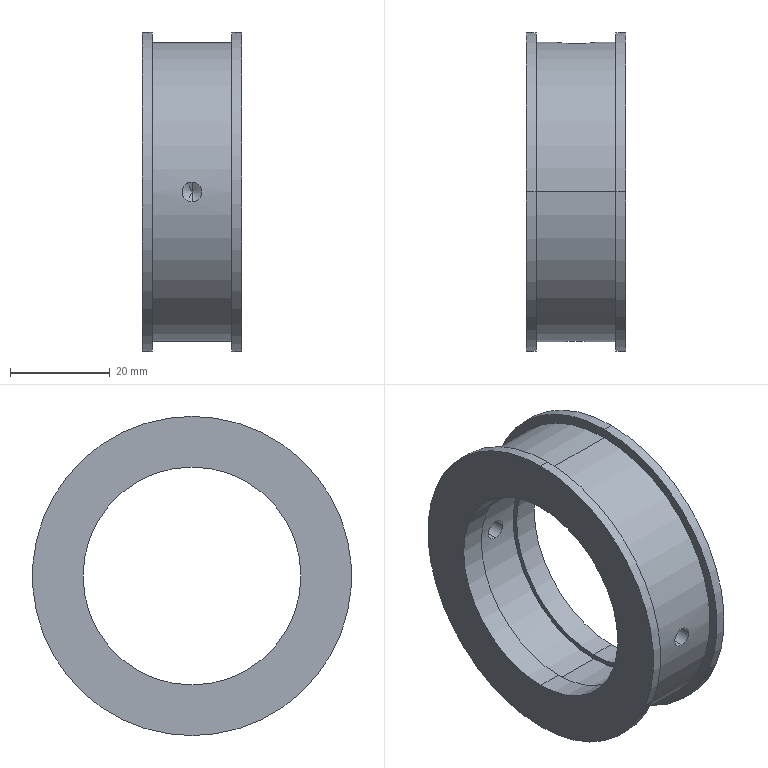Part | SolidWorks | features HoleWzd 3, Fillet 2, Revolution 1 | 1 solid | 31 faces | box 20 x 64 x 64 mm | volume 26515 mm3 | cylinder 18 | plane 7 | torus 2 | spline 2 | cone 2 | commonest cylinder face diameters 4 x4 43.7 x4 64 x4 7.5 x2 45.7 x2 60 x2
STEP:
#1=CARTESIAN_POINT('',(1.61,28.8,3.75));
#2=VERTEX_POINT('',#1);
#3=CARTESIAN_POINT('',(1.61,28.8,-3.75));
#4=VERTEX_POINT('',#3);
#5=CARTESIAN_POINT('',(1.61,28.8,0.));
#6=DIRECTION('',(0.,-1.,0.));
#7=DIRECTION('',(0.,0.,-1.));
#8=AXIS2_PLACEMENT_3D('',#5,#6,#7);
#9=CIRCLE('',#8,3.75);
#10=EDGE_CURVE('',#2,#4,#9,.T.);
#11=ORIENTED_EDGE('',*,*,#10,.F.);
#12=CARTESIAN_POINT('',(1.61,28.5,3.45));
#13=VERTEX_POINT('',#12);
#14=CARTESIAN_POINT('',(1.61,28.8,3.45));
#15=DIRECTION('',(1.,0.,0.));
#16=DIRECTION('',(0.,0.,-1.));
#17=AXIS2_PLACEMENT_3D('',#14,#15,#16);
#18=CIRCLE('',#17,0.3);
#19=EDGE_CURVE('',#2,#13,#18,.T.);
#20=ORIENTED_EDGE('',*,*,#19,.T.);
#21=CARTESIAN_POINT('',(1.61,28.5,-3.45));
#22=VERTEX_POINT('',#21);
#23=CARTESIAN_POINT('',(1.61,28.5,0.));
#24=DIRECTION('',(0.,1.,0.));
#25=DIRECTION('',(0.,0.,-1.));
#26=AXIS2_PLACEMENT_3D('',#23,#24,#25);
#27=CIRCLE('',#26,3.45);
#28=EDGE_CURVE('',#22,#13,#27,.T.);
#29=ORIENTED_EDGE('',*,*,#28,.F.);
#30=CARTESIAN_POINT('',(1.61,28.8,-3.45));
#31=DIRECTION('',(-1.,0.,0.));
#32=DIRECTION('',(0.,0.,1.));
#33=AXIS2_PLACEMENT_3D('',#30,#31,#32);
#34=CIRCLE('',#33,0.3);
#35=EDGE_CURVE('',#4,#22,#34,.T.);
#36=ORIENTED_EDGE('',*,*,#35,.F.);
#37=EDGE_LOOP('',(#11,#20,#29,#36));
#38=FACE_OUTER_BOUND('',#37,.T.);
#39=CARTESIAN_POINT('',(1.61,28.8,0.));
#40=DIRECTION('',(0.,-1.,0.));
#41=DIRECTION('',(0.,0.,-1.));
#42=AXIS2_PLACEMENT_3D('',#39,#40,#41);
#43=TOROIDAL_SURFACE('',#42,3.45,0.3);
#44=ADVANCED_FACE('',(#38),#43,.F.);
#45=CARTESIAN_POINT('',(0.7576,29.551,-3.652));
#46=VERTEX_POINT('',#45);
#47=CARTESIAN_POINT('',(1.61,29.537,3.75));
#48=VERTEX_POINT('',#47);
#49=CARTESIAN_POINT('',(0.7576,29.551,-3.652));
#50=CARTESIAN_POINT('',(0.5354,29.558,-3.6));
#51=CARTESIAN_POINT('',(0.3161,29.568,-3.527));
#52=CARTESIAN_POINT('',(-0.1007,29.591,-3.345));
#53=CARTESIAN_POINT('',(-0.2989,29.605,-3.236));
#54=CARTESIAN_POINT('',(-0.6749,29.634,-2.982));
#55=CARTESIAN_POINT('',(-0.8539,29.65,-2.836));
#56=CARTESIAN_POINT('',(-1.178,29.682,-2.518));
#57=CARTESIAN_POINT('',(-1.324,29.698,-2.346));
#58=CARTESIAN_POINT('',(-1.586,29.728,-1.974));
#59=CARTESIAN_POINT('',(-1.701,29.742,-1.774));
#60=CARTESIAN_POINT('',(-1.891,29.766,-1.363));
#61=CARTESIAN_POINT('',(-1.967,29.776,-1.149));
#62=CARTESIAN_POINT('',(-2.08,29.792,-0.7059));
#63=CARTESIAN_POINT('',(-2.116,29.797,-0.479));
#64=CARTESIAN_POINT('',(-2.146,29.801,-0.02683));
#65=CARTESIAN_POINT('',(-2.141,29.8,0.2003));
#66=CARTESIAN_POINT('',(-2.089,29.793,0.6567));
#67=CARTESIAN_POINT('',(-2.042,29.786,0.8794));
#68=CARTESIAN_POINT('',(-1.91,29.769,1.312));
#69=CARTESIAN_POINT('',(-1.823,29.757,1.524));
#70=CARTESIAN_POINT('',(-1.613,29.731,1.93));
#71=CARTESIAN_POINT('',(-1.491,29.717,2.121));
#72=CARTESIAN_POINT('',(-1.213,29.686,2.478));
#73=CARTESIAN_POINT('',(-1.056,29.67,2.647));
#74=CARTESIAN_POINT('',(-0.7163,29.638,2.95));
#75=CARTESIAN_POINT('',(-0.5345,29.623,3.084));
#76=CARTESIAN_POINT('',(-0.1474,29.594,3.32));
#77=CARTESIAN_POINT('',(0.06009,29.581,3.422));
#78=CARTESIAN_POINT('',(0.4848,29.56,3.584));
#79=CARTESIAN_POINT('',(0.7028,29.552,3.646));
#80=CARTESIAN_POINT('',(1.15,29.54,3.729));
#81=CARTESIAN_POINT('',(1.38,29.537,3.75));
#82=CARTESIAN_POINT('',(1.61,29.537,3.75));
#83=B_SPLINE_CURVE_WITH_KNOTS('',3,(#49,#50,#51,#52,#53,#54,#55,#56,#57,#58,#59,#60,#61,#62,#63,#64,#65,#66,#67,#68,#69,#70,#71,#72,#73,#74,#75,#76,#77,#78,#79,#80,#81,#82),.UNSPECIFIED.,.F.,.F.,(4,2,2,2,2,2,2,2,2,2,2,2,2,2,2,2,4),(0.01269,0.01337,0.01406,0.01474,0.01543,0.01611,0.0168,0.01748,0.01817,0.01885,0.01954,0.02022,0.02091,0.02159,0.02228,0.02296,0.02365),.UNSPECIFIED.);
#84=EDGE_CURVE('',#46,#48,#83,.T.);
#85=ORIENTED_EDGE('',*,*,#84,.F.);
#86=CARTESIAN_POINT('',(0.7121,29.749,-3.872));
#87=VERTEX_POINT('',#86);
#88=CARTESIAN_POINT('',(0.7121,29.551,-3.847));
#89=DIRECTION('',(-0.9734,0.02959,0.2273));
#90=DIRECTION('',(0.2274,0.,0.9738));
#91=AXIS2_PLACEMENT_3D('',#88,#89,#90);
#92=CIRCLE('',#91,0.2);
#93=EDGE_CURVE('',#46,#87,#92,.T.);
#94=ORIENTED_EDGE('',*,*,#93,.T.);
#95=CARTESIAN_POINT('',(2.509,29.749,3.872));
#96=VERTEX_POINT('',#95);
#97=CARTESIAN_POINT('',(2.509,29.749,3.872));
#98=CARTESIAN_POINT('',(2.254,29.741,3.932));
#99=CARTESIAN_POINT('',(1.996,29.737,3.966));
#100=CARTESIAN_POINT('',(1.474,29.734,3.983));
#101=CARTESIAN_POINT('',(1.21,29.737,3.965));
#102=CARTESIAN_POINT('',(0.6977,29.748,3.878));
#103=CARTESIAN_POINT('',(0.4487,29.757,3.81));
#104=CARTESIAN_POINT('',(-0.0351,29.78,3.624));
#105=CARTESIAN_POINT('',(-0.2706,29.795,3.506));
#106=CARTESIAN_POINT('',(-0.7071,29.826,3.231));
#107=CARTESIAN_POINT('',(-0.9108,29.843,3.072));
#108=CARTESIAN_POINT('',(-1.289,29.878,2.714));
#109=CARTESIAN_POINT('',(-1.459,29.895,2.517));
#110=CARTESIAN_POINT('',(-1.756,29.927,2.096));
#111=CARTESIAN_POINT('',(-1.886,29.943,1.869));
#112=CARTESIAN_POINT('',(-2.098,29.969,1.394));
#113=CARTESIAN_POINT('',(-2.18,29.979,1.149));
#114=CARTESIAN_POINT('',(-2.296,29.994,0.6447));
#115=CARTESIAN_POINT('',(-2.33,29.999,0.3829));
#116=CARTESIAN_POINT('',(-2.346,30.001,-0.135));
#117=CARTESIAN_POINT('',(-2.329,29.999,-0.3927));
#118=CARTESIAN_POINT('',(-2.245,29.987,-0.9056));
#119=CARTESIAN_POINT('',(-2.177,29.979,-1.16));
#120=CARTESIAN_POINT('',(-1.996,29.956,-1.643));
#121=CARTESIAN_POINT('',(-1.882,29.942,-1.876));
#122=CARTESIAN_POINT('',(-1.608,29.911,-2.321));
#123=CARTESIAN_POINT('',(-1.451,29.894,-2.526));
#124=CARTESIAN_POINT('',(-1.1,29.86,-2.904));
#125=CARTESIAN_POINT('',(-0.9038,29.842,-3.078));
#126=CARTESIAN_POINT('',(-0.4837,29.809,-3.382));
#127=CARTESIAN_POINT('',(-0.261,29.794,-3.512));
#128=CARTESIAN_POINT('',(0.2097,29.768,-3.727));
#129=CARTESIAN_POINT('',(0.4589,29.757,-3.813));
#130=CARTESIAN_POINT('',(0.7121,29.749,-3.872));
#131=B_SPLINE_CURVE_WITH_KNOTS('',3,(#97,#98,#99,#100,#101,#102,#103,#104,#105,#106,#107,#108,#109,#110,#111,#112,#113,#114,#115,#116,#117,#118,#119,#120,#121,#122,#123,#124,#125,#126,#127,#128,#129,#130),.UNSPECIFIED.,.F.,.F.,(4,2,2,2,2,2,2,2,2,2,2,2,2,2,2,2,4),(0.02421,0.025,0.02578,0.02657,0.02735,0.02814,0.02892,0.02971,0.03049,0.03128,0.03206,0.03285,0.03363,0.03442,0.0352,0.03599,0.03677),.UNSPECIFIED.);
#132=EDGE_CURVE('',#96,#87,#131,.T.);
#133=ORIENTED_EDGE('',*,*,#132,.F.);
#134=CARTESIAN_POINT('',(2.463,29.551,3.652));
#135=VERTEX_POINT('',#134);
#136=CARTESIAN_POINT('',(2.509,29.551,3.846));
#137=DIRECTION('',(0.9734,0.02959,-0.2273));
#138=DIRECTION('',(-0.2274,0.,-0.9738));
#139=AXIS2_PLACEMENT_3D('',#136,#137,#138);
#140=CIRCLE('',#139,0.2);
#141=EDGE_CURVE('',#135,#96,#140,.T.);
#142=ORIENTED_EDGE('',*,*,#141,.F.);
#143=CARTESIAN_POINT('',(1.61,29.537,3.75));
#144=CARTESIAN_POINT('',(1.754,29.537,3.75));
#145=CARTESIAN_POINT('',(2.041,29.539,3.733));
#146=CARTESIAN_POINT('',(2.323,29.546,3.684));
#147=CARTESIAN_POINT('',(2.463,29.551,3.652));
#148=B_SPLINE_CURVE_WITH_KNOTS('',3,(#143,#144,#145,#146,#147),.UNSPECIFIED.,.F.,.F.,(4,1,4),(0.,0.0004293,0.0008586),.UNSPECIFIED.);
#149=EDGE_CURVE('',#48,#135,#148,.T.);
#150=ORIENTED_EDGE('',*,*,#149,.F.);
#151=EDGE_LOOP('',(#85,#94,#133,#142,#150));
#152=FACE_OUTER_BOUND('',#151,.T.);
#153=CARTESIAN_POINT('',(2.463,29.551,3.652));
#154=CARTESIAN_POINT('',(2.457,29.778,3.653));
#155=CARTESIAN_POINT('',(2.509,29.749,3.872));
#156=CARTESIAN_POINT('',(2.222,29.543,3.708));
#157=CARTESIAN_POINT('',(2.216,29.771,3.709));
#158=CARTESIAN_POINT('',(2.254,29.741,3.932));
#159=CARTESIAN_POINT('',(1.979,29.538,3.74));
#160=CARTESIAN_POINT('',(1.976,29.767,3.74));
#161=CARTESIAN_POINT('',(1.998,29.737,3.966));
#162=CARTESIAN_POINT('',(1.49,29.536,3.756));
#163=CARTESIAN_POINT('',(1.491,29.765,3.756));
#164=CARTESIAN_POINT('',(1.484,29.734,3.983));
#165=CARTESIAN_POINT('',(1.241,29.539,3.74));
#166=CARTESIAN_POINT('',(1.245,29.767,3.74));
#167=CARTESIAN_POINT('',(1.222,29.737,3.966));
#168=CARTESIAN_POINT('',(0.7559,29.55,3.66));
#169=CARTESIAN_POINT('',(0.763,29.777,3.661));
#170=CARTESIAN_POINT('',(0.7104,29.748,3.881));
#171=CARTESIAN_POINT('',(0.5199,29.558,3.596));
#172=CARTESIAN_POINT('',(0.5288,29.784,3.599));
#173=CARTESIAN_POINT('',(0.4617,29.757,3.814));
#174=CARTESIAN_POINT('',(0.06088,29.581,3.424));
#175=CARTESIAN_POINT('',(0.07195,29.804,3.429));
#176=CARTESIAN_POINT('',(-0.02176,29.78,3.631));
#177=CARTESIAN_POINT('',(-0.1629,29.595,3.313));
#178=CARTESIAN_POINT('',(-0.151,29.817,3.32));
#179=CARTESIAN_POINT('',(-0.2575,29.794,3.513));
#180=CARTESIAN_POINT('',(-0.578,29.626,3.055));
#181=CARTESIAN_POINT('',(-0.5658,29.844,3.064));
#182=CARTESIAN_POINT('',(-0.6947,29.825,3.24));
#183=CARTESIAN_POINT('',(-0.772,29.643,2.907));
#184=CARTESIAN_POINT('',(-0.7601,29.859,2.916));
#185=CARTESIAN_POINT('',(-0.899,29.842,3.082));
#186=CARTESIAN_POINT('',(-1.132,29.677,2.57));
#187=CARTESIAN_POINT('',(-1.121,29.89,2.581));
#188=CARTESIAN_POINT('',(-1.278,29.877,2.725));
#189=CARTESIAN_POINT('',(-1.294,29.695,2.384));
#190=CARTESIAN_POINT('',(-1.285,29.905,2.396));
#191=CARTESIAN_POINT('',(-1.449,29.894,2.528));
#192=CARTESIAN_POINT('',(-1.579,29.727,1.988));
#193=CARTESIAN_POINT('',(-1.572,29.934,1.999));
#194=CARTESIAN_POINT('',(-1.749,29.927,2.108));
#195=CARTESIAN_POINT('',(-1.703,29.742,1.774));
#196=CARTESIAN_POINT('',(-1.697,29.948,1.785));
#197=CARTESIAN_POINT('',(-1.88,29.942,1.881));
#198=CARTESIAN_POINT('',(-1.907,29.768,1.325));
#199=CARTESIAN_POINT('',(-1.903,29.971,1.334));
#200=CARTESIAN_POINT('',(-2.094,29.968,1.405));
#201=CARTESIAN_POINT('',(-1.985,29.779,1.093));
#202=CARTESIAN_POINT('',(-1.983,29.981,1.101));
#203=CARTESIAN_POINT('',(-2.177,29.979,1.159));
#204=CARTESIAN_POINT('',(-2.097,29.794,0.6165));
#205=CARTESIAN_POINT('',(-2.096,29.995,0.6213));
#206=CARTESIAN_POINT('',(-2.294,29.994,0.6537));
#207=CARTESIAN_POINT('',(-2.13,29.799,0.3687));
#208=CARTESIAN_POINT('',(-2.129,29.999,0.3714));
#209=CARTESIAN_POINT('',(-2.329,29.999,0.391));
#210=CARTESIAN_POINT('',(-2.146,29.801,-0.1217));
#211=CARTESIAN_POINT('',(-2.146,30.001,-0.1225));
#212=CARTESIAN_POINT('',(-2.346,30.001,-0.129));
#213=CARTESIAN_POINT('',(-2.13,29.799,-0.3657));
#214=CARTESIAN_POINT('',(-2.13,29.999,-0.3686));
#215=CARTESIAN_POINT('',(-2.329,29.999,-0.3878));
#216=CARTESIAN_POINT('',(-2.05,29.788,-0.8512));
#217=CARTESIAN_POINT('',(-2.049,29.989,-0.8574));
#218=CARTESIAN_POINT('',(-2.245,29.988,-0.9027));
#219=CARTESIAN_POINT('',(-1.986,29.779,-1.092));
#220=CARTESIAN_POINT('',(-1.983,29.981,-1.1));
#221=CARTESIAN_POINT('',(-2.177,29.979,-1.158));
#222=CARTESIAN_POINT('',(-1.813,29.756,-1.549));
#223=CARTESIAN_POINT('',(-1.809,29.96,-1.559));
#224=CARTESIAN_POINT('',(-1.996,29.956,-1.643));
#225=CARTESIAN_POINT('',(-1.705,29.743,-1.769));
#226=CARTESIAN_POINT('',(-1.699,29.948,-1.78));
#227=CARTESIAN_POINT('',(-1.882,29.942,-1.876));
#228=CARTESIAN_POINT('',(-1.444,29.711,-2.189));
#229=CARTESIAN_POINT('',(-1.436,29.92,-2.201));
#230=CARTESIAN_POINT('',(-1.607,29.911,-2.322));
#231=CARTESIAN_POINT('',(-1.295,29.695,-2.383));
#232=CARTESIAN_POINT('',(-1.286,29.905,-2.395));
#233=CARTESIAN_POINT('',(-1.45,29.894,-2.527));
#234=CARTESIAN_POINT('',(-0.9616,29.661,-2.74));
#235=CARTESIAN_POINT('',(-0.9504,29.875,-2.751));
#236=CARTESIAN_POINT('',(-1.099,29.86,-2.905));
#237=CARTESIAN_POINT('',(-0.7748,29.643,-2.904));
#238=CARTESIAN_POINT('',(-0.7628,29.859,-2.914));
#239=CARTESIAN_POINT('',(-0.902,29.842,-3.08));
#240=CARTESIAN_POINT('',(-0.3759,29.61,-3.19));
#241=CARTESIAN_POINT('',(-0.3637,29.83,-3.198));
#242=CARTESIAN_POINT('',(-0.4819,29.809,-3.383));
#243=CARTESIAN_POINT('',(-0.1647,29.595,-3.312));
#244=CARTESIAN_POINT('',(-0.1528,29.817,-3.319));
#245=CARTESIAN_POINT('',(-0.2593,29.794,-3.512));
#246=CARTESIAN_POINT('',(0.2816,29.569,-3.515));
#247=CARTESIAN_POINT('',(0.2919,29.794,-3.519));
#248=CARTESIAN_POINT('',(0.2107,29.768,-3.728));
#249=CARTESIAN_POINT('',(0.5184,29.558,-3.596));
#250=CARTESIAN_POINT('',(0.5271,29.784,-3.598));
#251=CARTESIAN_POINT('',(0.4602,29.757,-3.813));
#252=CARTESIAN_POINT('',(0.7576,29.551,-3.652));
#253=CARTESIAN_POINT('',(0.7641,29.778,-3.653));
#254=CARTESIAN_POINT('',(0.7121,29.749,-3.872));
#255=(BOUNDED_SURFACE()B_SPLINE_SURFACE(3,2,((#153,#154,#155),(#156,#157,#158),(#159,#160,#161),(#162,#163,#164),(#165,#166,#167),(#168,#169,#170),(#171,#172,#173),(#174,#175,#176),(#177,#178,#179),(#180,#181,#182),(#183,#184,#185),(#186,#187,#188),(#189,#190,#191),(#192,#193,#194),(#195,#196,#197),(#198,#199,#200),(#201,#202,#203),(#204,#205,#206),(#207,#208,#209),(#210,#211,#212),(#213,#214,#215),(#216,#217,#218),(#219,#220,#221),(#222,#223,#224),(#225,#226,#227),(#228,#229,#230),(#231,#232,#233),(#234,#235,#236),(#237,#238,#239),(#240,#241,#242),(#243,#244,#245),(#246,#247,#248),(#249,#250,#251),(#252,#253,#254)),.UNSPECIFIED.,.F.,.F.,.F.)B_SPLINE_SURFACE_WITH_KNOTS((4,2,2,2,2,2,2,2,2,2,2,2,2,2,2,2,4),(3,3),(0.,0.0007725,0.001545,0.002318,0.00309,0.003863,0.004635,0.005408,0.00618,0.006953,0.007725,0.008498,0.00927,0.01004,0.01082,0.01159,0.01236),(0.,1.),.UNSPECIFIED.)GEOMETRIC_REPRESENTATION_ITEM()RATIONAL_B_SPLINE_SURFACE(((1.,0.6612,1.),(1.,0.6597,1.),(1.,0.6588,1.),(1.,0.6584,1.),(1.,0.6589,1.),(1.,0.661,1.),(1.,0.6626,1.),(1.,0.6669,1.),(1.,0.6696,1.),(1.,0.6754,1.),(1.,0.6785,1.),(1.,0.6849,1.),(1.,0.688,1.),(1.,0.694,1.),(1.,0.6967,1.),(1.,0.7014,1.),(1.,0.7033,1.),(1.,0.706,1.),(1.,0.7069,1.),(1.,0.7073,1.),(1.,0.7069,1.),(1.,0.7049,1.),(1.,0.7033,1.),(1.,0.6992,1.),(1.,0.6968,1.),(1.,0.6911,1.),(1.,0.688,1.),(1.,0.6817,1.),(1.,0.6785,1.),(1.,0.6724,1.),(1.,0.6696,1.),(1.,0.6647,1.),(1.,0.6626,1.),(1.,0.6612,1.)))REPRESENTATION_ITEM('')SURFACE());
#256=ADVANCED_FACE('',(#152),#255,.T.);
#257=CARTESIAN_POINT('',(1.61,-24.798,0.));
#258=VERTEX_POINT('',#257);
#259=CARTESIAN_POINT('',(1.61,-26.,-2.));
#260=VERTEX_POINT('',#259);
#261=CARTESIAN_POINT('',(1.61,-26.,-2.));
#262=DIRECTION('',(0.,-0.515,-0.8572));
#263=VECTOR('',#262,1000.);
#264=LINE('',#261,#263);
#265=EDGE_CURVE('',#258,#260,#264,.T.);
#266=ORIENTED_EDGE('',*,*,#265,.F.);
#267=CARTESIAN_POINT('',(1.61,-26.,2.));
#268=VERTEX_POINT('',#267);
#269=CARTESIAN_POINT('',(1.61,-26.,2.));
#270=DIRECTION('',(0.,-0.515,0.8572));
#271=VECTOR('',#270,1000.);
#272=LINE('',#269,#271);
#273=EDGE_CURVE('',#258,#268,#272,.T.);
#274=ORIENTED_EDGE('',*,*,#273,.T.);
#275=CARTESIAN_POINT('',(1.61,-26.,0.));
#276=DIRECTION('',(0.,-1.,0.));
#277=DIRECTION('',(0.,0.,-1.));
#278=AXIS2_PLACEMENT_3D('',#275,#276,#277);
#279=CIRCLE('',#278,2.);
#280=EDGE_CURVE('',#268,#260,#279,.T.);
#281=ORIENTED_EDGE('',*,*,#280,.T.);
#282=EDGE_LOOP('',(#266,#274,#281));
#283=FACE_OUTER_BOUND('',#282,.T.);
#284=CARTESIAN_POINT('',(1.61,-26.,0.));
#285=DIRECTION('',(0.,-1.,0.));
#286=DIRECTION('',(0.,0.,-1.));
#287=AXIS2_PLACEMENT_3D('',#284,#285,#286);
#288=CONICAL_SURFACE('',#287,2.,1.03);
#289=ADVANCED_FACE('',(#283),#288,.F.);
#290=ORIENTED_EDGE('',*,*,#280,.F.);
#291=CARTESIAN_POINT('',(1.61,-29.933,2.));
#292=VERTEX_POINT('',#291);
#293=CARTESIAN_POINT('',(1.61,-30.,2.));
#294=DIRECTION('',(0.,-1.,0.));
#295=VECTOR('',#294,1000.);
#296=LINE('',#293,#295);
#297=EDGE_CURVE('',#268,#292,#296,.T.);
#298=ORIENTED_EDGE('',*,*,#297,.T.);
#299=CARTESIAN_POINT('',(1.61,-29.933,-2.));
#300=VERTEX_POINT('',#299);
#301=CARTESIAN_POINT('',(1.61,-29.933,-2.));
#302=CARTESIAN_POINT('',(1.478,-29.933,-2.));
#303=CARTESIAN_POINT('',(1.348,-29.934,-1.987));
#304=CARTESIAN_POINT('',(1.093,-29.937,-1.936));
#305=CARTESIAN_POINT('',(0.9655,-29.94,-1.898));
#306=CARTESIAN_POINT('',(0.7232,-29.946,-1.797));
#307=CARTESIAN_POINT('',(0.6084,-29.95,-1.736));
#308=CARTESIAN_POINT('',(0.391,-29.958,-1.591));
#309=CARTESIAN_POINT('',(0.2881,-29.962,-1.506));
#310=CARTESIAN_POINT('',(0.01142,-29.975,-1.229));
#311=CARTESIAN_POINT('',(-0.1376,-29.984,-1.006));
#312=CARTESIAN_POINT('',(-0.337,-29.996,-0.525));
#313=CARTESIAN_POINT('',(-0.3896,-30.,-0.2617));
#314=CARTESIAN_POINT('',(-0.3897,-30.,0.1298));
#315=CARTESIAN_POINT('',(-0.3767,-29.999,0.2623));
#316=CARTESIAN_POINT('',(-0.3256,-29.996,0.5189));
#317=CARTESIAN_POINT('',(-0.2878,-29.993,0.6436));
#318=CARTESIAN_POINT('',(-0.1876,-29.987,0.8858));
#319=CARTESIAN_POINT('',(-0.125,-29.983,1.003));
#320=CARTESIAN_POINT('',(0.01983,-29.975,1.22));
#321=CARTESIAN_POINT('',(0.1025,-29.971,1.321));
#322=CARTESIAN_POINT('',(0.2892,-29.962,1.507));
#323=CARTESIAN_POINT('',(0.3903,-29.958,1.59));
#324=CARTESIAN_POINT('',(0.6069,-29.95,1.735));
#325=CARTESIAN_POINT('',(0.7238,-29.946,1.798));
#326=CARTESIAN_POINT('',(0.9662,-29.94,1.898));
#327=CARTESIAN_POINT('',(1.091,-29.937,1.936));
#328=CARTESIAN_POINT('',(1.347,-29.934,1.987));
#329=CARTESIAN_POINT('',(1.48,-29.933,2.));
#330=CARTESIAN_POINT('',(1.61,-29.933,2.));
#331=B_SPLINE_CURVE_WITH_KNOTS('',3,(#301,#302,#303,#304,#305,#306,#307,#308,#309,#310,#311,#312,#313,#314,#315,#316,#317,#318,#319,#320,#321,#322,#323,#324,#325,#326,#327,#328,#329,#330),.UNSPECIFIED.,.F.,.F.,(4,2,2,2,2,2,2,2,2,2,2,2,2,2,4),(0.,0.0003909,0.0007818,0.001173,0.001564,0.002345,0.003127,0.003518,0.003909,0.0043,0.004691,0.005082,0.005473,0.005864,0.006255),.UNSPECIFIED.);
#332=EDGE_CURVE('',#300,#292,#331,.T.);
#333=ORIENTED_EDGE('',*,*,#332,.F.);
#334=CARTESIAN_POINT('',(1.61,-30.,-2.));
#335=DIRECTION('',(0.,-1.,0.));
#336=VECTOR('',#335,1000.);
#337=LINE('',#334,#336);
#338=EDGE_CURVE('',#260,#300,#337,.T.);
#339=ORIENTED_EDGE('',*,*,#338,.F.);
#340=EDGE_LOOP('',(#290,#298,#333,#339));
#341=FACE_OUTER_BOUND('',#340,.T.);
#342=CARTESIAN_POINT('',(1.61,-30.,0.));
#343=DIRECTION('',(0.,-1.,0.));
#344=DIRECTION('',(0.,0.,-1.));
#345=AXIS2_PLACEMENT_3D('',#342,#343,#344);
#346=CYLINDRICAL_SURFACE('',#345,2.);
#347=ADVANCED_FACE('',(#341),#346,.F.);
#348=CARTESIAN_POINT('',(1.61,22.762,-2.));
#349=VERTEX_POINT('',#348);
#350=CARTESIAN_POINT('',(1.61,22.762,2.));
#351=VERTEX_POINT('',#350);
#352=CARTESIAN_POINT('',(1.61,22.762,-2.));
#353=CARTESIAN_POINT('',(1.349,22.762,-2.));
#354=CARTESIAN_POINT('',(1.086,22.767,-1.948));
#355=CARTESIAN_POINT('',(0.6047,22.783,-1.748));
#356=CARTESIAN_POINT('',(0.3816,22.795,-1.599));
#357=CARTESIAN_POINT('',(0.1049,22.812,-1.323));
#358=CARTESIAN_POINT('',(0.02038,22.818,-1.22));
#359=CARTESIAN_POINT('',(-0.1249,22.828,-1.003));
#360=CARTESIAN_POINT('',(-0.1864,22.833,-0.8882));
#361=CARTESIAN_POINT('',(-0.2869,22.841,-0.6463));
#362=CARTESIAN_POINT('',(-0.3255,22.844,-0.5192));
#363=CARTESIAN_POINT('',(-0.3765,22.849,-0.2635));
#364=CARTESIAN_POINT('',(-0.3896,22.85,-0.1336));
#365=CARTESIAN_POINT('',(-0.3898,22.85,0.1305));
#366=CARTESIAN_POINT('',(-0.3769,22.849,0.2608));
#367=CARTESIAN_POINT('',(-0.3262,22.845,0.5164));
#368=CARTESIAN_POINT('',(-0.2879,22.841,0.6434));
#369=CARTESIAN_POINT('',(-0.1876,22.833,0.8857));
#370=CARTESIAN_POINT('',(-0.1263,22.828,1.001));
#371=CARTESIAN_POINT('',(0.01862,22.818,1.218));
#372=CARTESIAN_POINT('',(0.103,22.812,1.321));
#373=CARTESIAN_POINT('',(0.3795,22.795,1.598));
#374=CARTESIAN_POINT('',(0.6023,22.783,1.747));
#375=CARTESIAN_POINT('',(1.083,22.767,1.947));
#376=CARTESIAN_POINT('',(1.346,22.762,2.));
#377=CARTESIAN_POINT('',(1.61,22.762,2.));
#378=B_SPLINE_CURVE_WITH_KNOTS('',3,(#352,#353,#354,#355,#356,#357,#358,#359,#360,#361,#362,#363,#364,#365,#366,#367,#368,#369,#370,#371,#372,#373,#374,#375,#376,#377),.UNSPECIFIED.,.F.,.F.,(4,2,2,2,2,2,2,2,2,2,2,2,4),(0.006256,0.007038,0.00782,0.00821,0.008601,0.008992,0.009383,0.009774,0.01016,0.01056,0.01095,0.01173,0.01251),.UNSPECIFIED.);
#379=EDGE_CURVE('',#349,#351,#378,.T.);
#380=ORIENTED_EDGE('',*,*,#379,.F.);
#381=CARTESIAN_POINT('',(1.61,28.5,-2.));
#382=VERTEX_POINT('',#381);
#383=CARTESIAN_POINT('',(1.61,28.5,-2.));
#384=DIRECTION('',(0.,1.,0.));
#385=VECTOR('',#384,1000.);
#386=LINE('',#383,#385);
#387=EDGE_CURVE('',#349,#382,#386,.T.);
#388=ORIENTED_EDGE('',*,*,#387,.T.);
#389=CARTESIAN_POINT('',(1.61,28.5,2.));
#390=VERTEX_POINT('',#389);
#391=CARTESIAN_POINT('',(1.61,28.5,0.));
#392=DIRECTION('',(0.,1.,0.));
#393=DIRECTION('',(0.,0.,1.));
#394=AXIS2_PLACEMENT_3D('',#391,#392,#393);
#395=CIRCLE('',#394,2.);
#396=EDGE_CURVE('',#382,#390,#395,.T.);
#397=ORIENTED_EDGE('',*,*,#396,.T.);
#398=CARTESIAN_POINT('',(1.61,28.5,2.));
#399=DIRECTION('',(0.,1.,0.));
#400=VECTOR('',#399,1000.);
#401=LINE('',#398,#400);
#402=EDGE_CURVE('',#351,#390,#401,.T.);
#403=ORIENTED_EDGE('',*,*,#402,.F.);
#404=EDGE_LOOP('',(#380,#388,#397,#403));
#405=FACE_OUTER_BOUND('',#404,.T.);
#406=CARTESIAN_POINT('',(1.61,28.5,0.));
#407=DIRECTION('',(0.,1.,0.));
#408=DIRECTION('',(0.,0.,1.));
#409=AXIS2_PLACEMENT_3D('',#406,#407,#408);
#410=CYLINDRICAL_SURFACE('',#409,2.);
#411=ADVANCED_FACE('',(#405),#410,.F.);
#412=ORIENTED_EDGE('',*,*,#10,.T.);
#413=CARTESIAN_POINT('',(1.61,29.537,-3.75));
#414=VERTEX_POINT('',#413);
#415=CARTESIAN_POINT('',(1.61,30.,-3.75));
#416=DIRECTION('',(0.,1.,0.));
#417=VECTOR('',#416,1000.);
#418=LINE('',#415,#417);
#419=EDGE_CURVE('',#4,#414,#418,.T.);
#420=ORIENTED_EDGE('',*,*,#419,.T.);
#421=CARTESIAN_POINT('',(1.61,29.537,-3.75));
#422=CARTESIAN_POINT('',(1.468,29.537,-3.75));
#423=CARTESIAN_POINT('',(1.325,29.538,-3.742));
#424=CARTESIAN_POINT('',(1.038,29.543,-3.709));
#425=CARTESIAN_POINT('',(0.8971,29.546,-3.684));
#426=CARTESIAN_POINT('',(0.7576,29.551,-3.652));
#427=B_SPLINE_CURVE_WITH_KNOTS('',3,(#421,#422,#423,#424,#425,#426),.UNSPECIFIED.,.F.,.F.,(4,2,4),(0.01183,0.01226,0.01269),.UNSPECIFIED.);
#428=EDGE_CURVE('',#414,#46,#427,.T.);
#429=ORIENTED_EDGE('',*,*,#428,.T.);
#430=ORIENTED_EDGE('',*,*,#84,.T.);
#431=CARTESIAN_POINT('',(1.61,30.,3.75));
#432=DIRECTION('',(0.,1.,0.));
#433=VECTOR('',#432,1000.);
#434=LINE('',#431,#433);
#435=EDGE_CURVE('',#2,#48,#434,.T.);
#436=ORIENTED_EDGE('',*,*,#435,.F.);
#437=EDGE_LOOP('',(#412,#420,#429,#430,#436));
#438=FACE_OUTER_BOUND('',#437,.T.);
#439=CARTESIAN_POINT('',(1.61,30.,0.));
#440=DIRECTION('',(0.,1.,0.));
#441=DIRECTION('',(0.,0.,1.));
#442=AXIS2_PLACEMENT_3D('',#439,#440,#441);
#443=CYLINDRICAL_SURFACE('',#442,3.75);
#444=ADVANCED_FACE('',(#438),#443,.F.);
#445=CARTESIAN_POINT('',(-3.39,0.,-21.85));
#446=VERTEX_POINT('',#445);
#447=CARTESIAN_POINT('',(-3.39,0.,21.85));
#448=VERTEX_POINT('',#447);
#449=CARTESIAN_POINT('',(-3.39,0.,0.));
#450=DIRECTION('',(-1.,0.,0.));
#451=DIRECTION('',(0.,0.,1.));
#452=AXIS2_PLACEMENT_3D('',#449,#450,#451);
#453=CIRCLE('',#452,21.85);
#454=EDGE_CURVE('',#446,#448,#453,.T.);
#455=ORIENTED_EDGE('',*,*,#454,.F.);
#456=CARTESIAN_POINT('',(-8.39,0.,-21.85));
#457=VERTEX_POINT('',#456);
#458=CARTESIAN_POINT('',(-19.037,0.,-21.85));
#459=DIRECTION('',(-1.,0.,0.));
#460=VECTOR('',#459,1000.);
#461=LINE('',#458,#460);
#462=EDGE_CURVE('',#446,#457,#461,.T.);
#463=ORIENTED_EDGE('',*,*,#462,.T.);
#464=CARTESIAN_POINT('',(-8.39,0.,21.85));
#465=VERTEX_POINT('',#464);
#466=CARTESIAN_POINT('',(-8.39,0.,0.));
#467=DIRECTION('',(-1.,0.,0.));
#468=DIRECTION('',(0.,0.,1.));
#469=AXIS2_PLACEMENT_3D('',#466,#467,#468);
#470=CIRCLE('',#469,21.85);
#471=EDGE_CURVE('',#457,#465,#470,.T.);
#472=ORIENTED_EDGE('',*,*,#471,.T.);
#473=CARTESIAN_POINT('',(-19.037,0.,21.85));
#474=DIRECTION('',(-1.,0.,0.));
#475=VECTOR('',#474,1000.);
#476=LINE('',#473,#475);
#477=EDGE_CURVE('',#448,#465,#476,.T.);
#478=ORIENTED_EDGE('',*,*,#477,.F.);
#479=EDGE_LOOP('',(#455,#463,#472,#478));
#480=FACE_OUTER_BOUND('',#479,.T.);
#481=CARTESIAN_POINT('',(-19.037,0.,0.));
#482=DIRECTION('',(-1.,0.,0.));
#483=DIRECTION('',(0.,0.,1.));
#484=AXIS2_PLACEMENT_3D('',#481,#482,#483);
#485=CYLINDRICAL_SURFACE('',#484,21.85);
#486=ADVANCED_FACE('',(#480),#485,.F.);
#487=CARTESIAN_POINT('',(6.61,0.,-22.85));
#488=VERTEX_POINT('',#487);
#489=CARTESIAN_POINT('',(6.61,0.,22.85));
#490=VERTEX_POINT('',#489);
#491=CARTESIAN_POINT('',(6.61,0.,0.));
#492=DIRECTION('',(-1.,0.,0.));
#493=DIRECTION('',(0.,0.,1.));
#494=AXIS2_PLACEMENT_3D('',#491,#492,#493);
#495=CIRCLE('',#494,22.85);
#496=EDGE_CURVE('',#488,#490,#495,.T.);
#497=ORIENTED_EDGE('',*,*,#496,.F.);
#498=CARTESIAN_POINT('',(-3.39,0.,-22.85));
#499=VERTEX_POINT('',#498);
#500=CARTESIAN_POINT('',(-19.037,0.,-22.85));
#501=DIRECTION('',(-1.,0.,0.));
#502=VECTOR('',#501,1000.);
#503=LINE('',#500,#502);
#504=EDGE_CURVE('',#488,#499,#503,.T.);
#505=ORIENTED_EDGE('',*,*,#504,.T.);
#506=CARTESIAN_POINT('',(-3.39,0.,22.85));
#507=VERTEX_POINT('',#506);
#508=CARTESIAN_POINT('',(-3.39,0.,0.));
#509=DIRECTION('',(-1.,0.,0.));
#510=DIRECTION('',(0.,0.,1.));
#511=AXIS2_PLACEMENT_3D('',#508,#509,#510);
#512=CIRCLE('',#511,22.85);
#513=EDGE_CURVE('',#499,#507,#512,.T.);
#514=ORIENTED_EDGE('',*,*,#513,.T.);
#515=CARTESIAN_POINT('',(-19.037,0.,22.85));
#516=DIRECTION('',(-1.,0.,0.));
#517=VECTOR('',#516,1000.);
#518=LINE('',#515,#517);
#519=EDGE_CURVE('',#490,#507,#518,.T.);
#520=ORIENTED_EDGE('',*,*,#519,.F.);
#521=EDGE_LOOP('',(#497,#505,#514,#520));
#522=FACE_OUTER_BOUND('',#521,.T.);
#523=CARTESIAN_POINT('',(-19.037,0.,0.));
#524=DIRECTION('',(-1.,0.,0.));
#525=DIRECTION('',(0.,0.,1.));
#526=AXIS2_PLACEMENT_3D('',#523,#524,#525);
#527=CYLINDRICAL_SURFACE('',#526,22.85);
#528=ADVANCED_FACE('',(#522),#527,.F.);
#529=CARTESIAN_POINT('',(11.61,0.,-21.85));
#530=VERTEX_POINT('',#529);
#531=CARTESIAN_POINT('',(11.61,0.,21.85));
#532=VERTEX_POINT('',#531);
#533=CARTESIAN_POINT('',(11.61,0.,0.));
#534=DIRECTION('',(-1.,0.,0.));
#535=DIRECTION('',(0.,0.,1.));
#536=AXIS2_PLACEMENT_3D('',#533,#534,#535);
#537=CIRCLE('',#536,21.85);
#538=EDGE_CURVE('',#530,#532,#537,.T.);
#539=ORIENTED_EDGE('',*,*,#538,.F.);
#540=CARTESIAN_POINT('',(6.61,0.,-21.85));
#541=VERTEX_POINT('',#540);
#542=CARTESIAN_POINT('',(-19.037,0.,-21.85));
#543=DIRECTION('',(-1.,0.,0.));
#544=VECTOR('',#543,1000.);
#545=LINE('',#542,#544);
#546=EDGE_CURVE('',#530,#541,#545,.T.);
#547=ORIENTED_EDGE('',*,*,#546,.T.);
#548=CARTESIAN_POINT('',(6.61,0.,21.85));
#549=VERTEX_POINT('',#548);
#550=CARTESIAN_POINT('',(6.61,0.,0.));
#551=DIRECTION('',(-1.,0.,0.));
#552=DIRECTION('',(0.,0.,1.));
#553=AXIS2_PLACEMENT_3D('',#550,#551,#552);
#554=CIRCLE('',#553,21.85);
#555=EDGE_CURVE('',#541,#549,#554,.T.);
#556=ORIENTED_EDGE('',*,*,#555,.T.);
#557=CARTESIAN_POINT('',(-19.037,0.,21.85));
#558=DIRECTION('',(-1.,0.,0.));
#559=VECTOR('',#558,1000.);
#560=LINE('',#557,#559);
#561=EDGE_CURVE('',#532,#549,#560,.T.);
#562=ORIENTED_EDGE('',*,*,#561,.F.);
#563=EDGE_LOOP('',(#539,#547,#556,#562));
#564=FACE_OUTER_BOUND('',#563,.T.);
#565=CARTESIAN_POINT('',(-19.037,0.,0.));
#566=DIRECTION('',(-1.,0.,0.));
#567=DIRECTION('',(0.,0.,1.));
#568=AXIS2_PLACEMENT_3D('',#565,#566,#567);
#569=CYLINDRICAL_SURFACE('',#568,21.85);
#570=ADVANCED_FACE('',(#564),#569,.F.);
#571=CARTESIAN_POINT('',(11.61,0.,32.));
#572=VERTEX_POINT('',#571);
#573=CARTESIAN_POINT('',(11.61,0.,-32.));
#574=VERTEX_POINT('',#573);
#575=CARTESIAN_POINT('',(11.61,0.,0.));
#576=DIRECTION('',(-1.,0.,0.));
#577=DIRECTION('',(0.,0.,1.));
#578=AXIS2_PLACEMENT_3D('',#575,#576,#577);
#579=CIRCLE('',#578,32.);
#580=EDGE_CURVE('',#572,#574,#579,.T.);
#581=ORIENTED_EDGE('',*,*,#580,.T.);
#582=CARTESIAN_POINT('',(9.61,0.,-32.));
#583=VERTEX_POINT('',#582);
#584=CARTESIAN_POINT('',(-19.037,0.,-32.));
#585=DIRECTION('',(-1.,0.,0.));
#586=VECTOR('',#585,1000.);
#587=LINE('',#584,#586);
#588=EDGE_CURVE('',#574,#583,#587,.T.);
#589=ORIENTED_EDGE('',*,*,#588,.T.);
#590=CARTESIAN_POINT('',(9.61,0.,32.));
#591=VERTEX_POINT('',#590);
#592=CARTESIAN_POINT('',(9.61,0.,0.));
#593=DIRECTION('',(-1.,0.,0.));
#594=DIRECTION('',(0.,0.,1.));
#595=AXIS2_PLACEMENT_3D('',#592,#593,#594);
#596=CIRCLE('',#595,32.);
#597=EDGE_CURVE('',#591,#583,#596,.T.);
#598=ORIENTED_EDGE('',*,*,#597,.F.);
#599=CARTESIAN_POINT('',(-19.037,0.,32.));
#600=DIRECTION('',(-1.,0.,0.));
#601=VECTOR('',#600,1000.);
#602=LINE('',#599,#601);
#603=EDGE_CURVE('',#572,#591,#602,.T.);
#604=ORIENTED_EDGE('',*,*,#603,.F.);
#605=EDGE_LOOP('',(#581,#589,#598,#604));
#606=FACE_OUTER_BOUND('',#605,.T.);
#607=CARTESIAN_POINT('',(-19.037,0.,0.));
#608=DIRECTION('',(-1.,0.,0.));
#609=DIRECTION('',(0.,0.,1.));
#610=AXIS2_PLACEMENT_3D('',#607,#608,#609);
#611=CYLINDRICAL_SURFACE('',#610,32.);
#612=ADVANCED_FACE('',(#606),#611,.T.);
#613=ORIENTED_EDGE('',*,*,#132,.T.);
#614=CARTESIAN_POINT('',(0.7121,29.749,-3.872));
#615=CARTESIAN_POINT('',(0.9654,29.741,-3.932));
#616=CARTESIAN_POINT('',(1.227,29.737,-3.966));
#617=CARTESIAN_POINT('',(1.746,29.734,-3.983));
#618=CARTESIAN_POINT('',(2.003,29.737,-3.965));
#619=CARTESIAN_POINT('',(2.516,29.748,-3.879));
#620=CARTESIAN_POINT('',(2.77,29.757,-3.81));
#621=CARTESIAN_POINT('',(3.253,29.78,-3.626));
#622=CARTESIAN_POINT('',(3.484,29.794,-3.51));
#623=CARTESIAN_POINT('',(3.927,29.826,-3.232));
#624=CARTESIAN_POINT('',(4.131,29.843,-3.073));
#625=CARTESIAN_POINT('',(4.505,29.877,-2.718));
#626=CARTESIAN_POINT('',(4.677,29.895,-2.519));
#627=CARTESIAN_POINT('',(4.977,29.927,-2.096));
#628=CARTESIAN_POINT('',(5.105,29.942,-1.872));
#629=CARTESIAN_POINT('',(5.317,29.968,-1.399));
#630=CARTESIAN_POINT('',(5.401,29.979,-1.149));
#631=CARTESIAN_POINT('',(5.517,29.994,-0.6445));
#632=CARTESIAN_POINT('',(5.55,29.999,-0.3881));
#633=CARTESIAN_POINT('',(5.567,30.001,0.1335));
#634=CARTESIAN_POINT('',(5.549,29.998,0.3946));
#635=CARTESIAN_POINT('',(5.465,29.987,0.9045));
#636=CARTESIAN_POINT('',(5.398,29.979,1.157));
#637=CARTESIAN_POINT('',(5.216,29.956,1.646));
#638=CARTESIAN_POINT('',(5.102,29.942,1.877));
#639=CARTESIAN_POINT('',(4.831,29.911,2.317));
#640=CARTESIAN_POINT('',(4.671,29.894,2.527));
#641=CARTESIAN_POINT('',(4.319,29.86,2.906));
#642=CARTESIAN_POINT('',(4.126,29.842,3.077));
#643=CARTESIAN_POINT('',(3.705,29.809,3.381));
#644=CARTESIAN_POINT('',(3.478,29.794,3.514));
#645=CARTESIAN_POINT('',(3.008,29.768,3.728));
#646=CARTESIAN_POINT('',(2.764,29.757,3.812));
#647=CARTESIAN_POINT('',(2.509,29.749,3.872));
#648=B_SPLINE_CURVE_WITH_KNOTS('',3,(#614,#615,#616,#617,#618,#619,#620,#621,#622,#623,#624,#625,#626,#627,#628,#629,#630,#631,#632,#633,#634,#635,#636,#637,#638,#639,#640,#641,#642,#643,#644,#645,#646,#647),.UNSPECIFIED.,.F.,.F.,(4,2,2,2,2,2,2,2,2,2,2,2,2,2,2,2,4),(0.01165,0.01243,0.01322,0.014,0.01479,0.01557,0.01636,0.01714,0.01793,0.01872,0.0195,0.02029,0.02107,0.02186,0.02264,0.02343,0.02421),.UNSPECIFIED.);
#649=EDGE_CURVE('',#87,#96,#648,.T.);
#650=ORIENTED_EDGE('',*,*,#649,.T.);
#651=EDGE_LOOP('',(#613,#650));
#652=FACE_BOUND('',#651,.T.);
#653=CARTESIAN_POINT('',(9.61,0.,30.));
#654=VERTEX_POINT('',#653);
#655=CARTESIAN_POINT('',(9.61,0.,-30.));
#656=VERTEX_POINT('',#655);
#657=CARTESIAN_POINT('',(9.61,0.,0.));
#658=DIRECTION('',(-1.,0.,0.));
#659=DIRECTION('',(0.,0.,1.));
#660=AXIS2_PLACEMENT_3D('',#657,#658,#659);
#661=CIRCLE('',#660,30.);
#662=EDGE_CURVE('',#654,#656,#661,.T.);
#663=ORIENTED_EDGE('',*,*,#662,.T.);
#664=CARTESIAN_POINT('',(-6.39,0.,-30.));
#665=VERTEX_POINT('',#664);
#666=CARTESIAN_POINT('',(-19.037,0.,-30.));
#667=DIRECTION('',(-1.,0.,0.));
#668=VECTOR('',#667,1000.);
#669=LINE('',#666,#668);
#670=EDGE_CURVE('',#656,#665,#669,.T.);
#671=ORIENTED_EDGE('',*,*,#670,.T.);
#672=CARTESIAN_POINT('',(-6.39,0.,30.));
#673=VERTEX_POINT('',#672);
#674=CARTESIAN_POINT('',(-6.39,0.,0.));
#675=DIRECTION('',(-1.,0.,0.));
#676=DIRECTION('',(0.,0.,1.));
#677=AXIS2_PLACEMENT_3D('',#674,#675,#676);
#678=CIRCLE('',#677,30.);
#679=EDGE_CURVE('',#673,#665,#678,.T.);
#680=ORIENTED_EDGE('',*,*,#679,.F.);
#681=CARTESIAN_POINT('',(-19.037,0.,30.));
#682=DIRECTION('',(-1.,0.,0.));
#683=VECTOR('',#682,1000.);
#684=LINE('',#681,#683);
#685=EDGE_CURVE('',#654,#673,#684,.T.);
#686=ORIENTED_EDGE('',*,*,#685,.F.);
#687=EDGE_LOOP('',(#663,#671,#680,#686));
#688=FACE_OUTER_BOUND('',#687,.T.);
#689=CARTESIAN_POINT('',(-19.037,0.,0.));
#690=DIRECTION('',(-1.,0.,0.));
#691=DIRECTION('',(0.,0.,1.));
#692=AXIS2_PLACEMENT_3D('',#689,#690,#691);
#693=CYLINDRICAL_SURFACE('',#692,30.);
#694=ADVANCED_FACE('',(#652,#688),#693,.T.);
#695=CARTESIAN_POINT('',(-6.39,0.,32.));
#696=VERTEX_POINT('',#695);
#697=CARTESIAN_POINT('',(-6.39,0.,-32.));
#698=VERTEX_POINT('',#697);
#699=CARTESIAN_POINT('',(-6.39,0.,0.));
#700=DIRECTION('',(-1.,0.,0.));
#701=DIRECTION('',(0.,0.,1.));
#702=AXIS2_PLACEMENT_3D('',#699,#700,#701);
#703=CIRCLE('',#702,32.);
#704=EDGE_CURVE('',#696,#698,#703,.T.);
#705=ORIENTED_EDGE('',*,*,#704,.T.);
#706=CARTESIAN_POINT('',(-8.39,0.,-32.));
#707=VERTEX_POINT('',#706);
#708=CARTESIAN_POINT('',(-19.037,0.,-32.));
#709=DIRECTION('',(-1.,0.,0.));
#710=VECTOR('',#709,1000.);
#711=LINE('',#708,#710);
#712=EDGE_CURVE('',#698,#707,#711,.T.);
#713=ORIENTED_EDGE('',*,*,#712,.T.);
#714=CARTESIAN_POINT('',(-8.39,0.,32.));
#715=VERTEX_POINT('',#714);
#716=CARTESIAN_POINT('',(-8.39,0.,0.));
#717=DIRECTION('',(-1.,0.,0.));
#718=DIRECTION('',(0.,0.,1.));
#719=AXIS2_PLACEMENT_3D('',#716,#717,#718);
#720=CIRCLE('',#719,32.);
#721=EDGE_CURVE('',#715,#707,#720,.T.);
#722=ORIENTED_EDGE('',*,*,#721,.F.);
#723=CARTESIAN_POINT('',(-19.037,0.,32.));
#724=DIRECTION('',(-1.,0.,0.));
#725=VECTOR('',#724,1000.);
#726=LINE('',#723,#725);
#727=EDGE_CURVE('',#696,#715,#726,.T.);
#728=ORIENTED_EDGE('',*,*,#727,.F.);
#729=EDGE_LOOP('',(#705,#713,#722,#728));
#730=FACE_OUTER_BOUND('',#729,.T.);
#731=CARTESIAN_POINT('',(-19.037,0.,0.));
#732=DIRECTION('',(-1.,0.,0.));
#733=DIRECTION('',(0.,0.,1.));
#734=AXIS2_PLACEMENT_3D('',#731,#732,#733);
#735=CYLINDRICAL_SURFACE('',#734,32.);
#736=ADVANCED_FACE('',(#730),#735,.T.);
#737=ORIENTED_EDGE('',*,*,#712,.F.);
#738=CARTESIAN_POINT('',(-6.39,0.,0.));
#739=DIRECTION('',(-1.,0.,0.));
#740=DIRECTION('',(0.,0.,1.));
#741=AXIS2_PLACEMENT_3D('',#738,#739,#740);
#742=CIRCLE('',#741,32.);
#743=EDGE_CURVE('',#698,#696,#742,.T.);
#744=ORIENTED_EDGE('',*,*,#743,.T.);
#745=ORIENTED_EDGE('',*,*,#727,.T.);
#746=CARTESIAN_POINT('',(-8.39,0.,0.));
#747=DIRECTION('',(-1.,0.,0.));
#748=DIRECTION('',(0.,0.,1.));
#749=AXIS2_PLACEMENT_3D('',#746,#747,#748);
#750=CIRCLE('',#749,32.);
#751=EDGE_CURVE('',#707,#715,#750,.T.);
#752=ORIENTED_EDGE('',*,*,#751,.F.);
#753=EDGE_LOOP('',(#737,#744,#745,#752));
#754=FACE_OUTER_BOUND('',#753,.T.);
#755=CARTESIAN_POINT('',(-19.037,0.,0.));
#756=DIRECTION('',(-1.,0.,0.));
#757=DIRECTION('',(0.,0.,1.));
#758=AXIS2_PLACEMENT_3D('',#755,#756,#757);
#759=CYLINDRICAL_SURFACE('',#758,32.);
#760=ADVANCED_FACE('',(#754),#759,.T.);
#761=ORIENTED_EDGE('',*,*,#704,.F.);
#762=ORIENTED_EDGE('',*,*,#743,.F.);
#763=EDGE_LOOP('',(#761,#762));
#764=FACE_OUTER_BOUND('',#763,.T.);
#765=ORIENTED_EDGE('',*,*,#679,.T.);
#766=CARTESIAN_POINT('',(-6.39,0.,0.));
#767=DIRECTION('',(-1.,0.,0.));
#768=DIRECTION('',(0.,0.,1.));
#769=AXIS2_PLACEMENT_3D('',#766,#767,#768);
#770=CIRCLE('',#769,30.);
#771=EDGE_CURVE('',#665,#673,#770,.T.);
#772=ORIENTED_EDGE('',*,*,#771,.T.);
#773=EDGE_LOOP('',(#765,#772));
#774=FACE_BOUND('',#773,.T.);
#775=CARTESIAN_POINT('',(-6.39,32.,0.));
#776=DIRECTION('',(-1.,0.,0.));
#777=DIRECTION('',(0.,0.,1.));
#778=AXIS2_PLACEMENT_3D('',#775,#776,#777);
#779=PLANE('',#778);
#780=ADVANCED_FACE('',(#764,#774),#779,.F.);
#781=ORIENTED_EDGE('',*,*,#670,.F.);
#782=CARTESIAN_POINT('',(9.61,0.,0.));
#783=DIRECTION('',(-1.,0.,0.));
#784=DIRECTION('',(0.,0.,1.));
#785=AXIS2_PLACEMENT_3D('',#782,#783,#784);
#786=CIRCLE('',#785,30.);
#787=EDGE_CURVE('',#656,#654,#786,.T.);
#788=ORIENTED_EDGE('',*,*,#787,.T.);
#789=ORIENTED_EDGE('',*,*,#685,.T.);
#790=ORIENTED_EDGE('',*,*,#771,.F.);
#791=EDGE_LOOP('',(#781,#788,#789,#790));
#792=FACE_OUTER_BOUND('',#791,.T.);
#793=ORIENTED_EDGE('',*,*,#332,.T.);
#794=CARTESIAN_POINT('',(1.61,-29.933,2.));
#795=CARTESIAN_POINT('',(1.871,-29.933,2.));
#796=CARTESIAN_POINT('',(2.135,-29.937,1.948));
#797=CARTESIAN_POINT('',(2.616,-29.949,1.748));
#798=CARTESIAN_POINT('',(2.839,-29.958,1.599));
#799=CARTESIAN_POINT('',(3.116,-29.971,1.323));
#800=CARTESIAN_POINT('',(3.2,-29.975,1.22));
#801=CARTESIAN_POINT('',(3.346,-29.983,1.003));
#802=CARTESIAN_POINT('',(3.407,-29.987,0.8881));
#803=CARTESIAN_POINT('',(3.508,-29.993,0.6462));
#804=CARTESIAN_POINT('',(3.546,-29.996,0.5191));
#805=CARTESIAN_POINT('',(3.597,-29.999,0.2635));
#806=CARTESIAN_POINT('',(3.61,-30.,0.1336));
#807=CARTESIAN_POINT('',(3.61,-30.,-0.1304));
#808=CARTESIAN_POINT('',(3.598,-29.999,-0.2607));
#809=CARTESIAN_POINT('',(3.547,-29.996,-0.5163));
#810=CARTESIAN_POINT('',(3.509,-29.993,-0.6432));
#811=CARTESIAN_POINT('',(3.408,-29.987,-0.8857));
#812=CARTESIAN_POINT('',(3.347,-29.984,-1.001));
#813=CARTESIAN_POINT('',(3.202,-29.975,-1.218));
#814=CARTESIAN_POINT('',(3.118,-29.971,-1.321));
#815=CARTESIAN_POINT('',(2.933,-29.962,-1.506));
#816=CARTESIAN_POINT('',(2.833,-29.958,-1.588));
#817=CARTESIAN_POINT('',(2.615,-29.95,-1.735));
#818=CARTESIAN_POINT('',(2.498,-29.946,-1.797));
#819=CARTESIAN_POINT('',(2.137,-29.937,-1.947));
#820=CARTESIAN_POINT('',(1.875,-29.933,-2.));
#821=CARTESIAN_POINT('',(1.61,-29.933,-2.));
#822=B_SPLINE_CURVE_WITH_KNOTS('',3,(#794,#795,#796,#797,#798,#799,#800,#801,#802,#803,#804,#805,#806,#807,#808,#809,#810,#811,#812,#813,#814,#815,#816,#817,#818,#819,#820,#821),.UNSPECIFIED.,.F.,.F.,(4,2,2,2,2,2,2,2,2,2,2,2,2,4),(0.006255,0.007036,0.007818,0.008209,0.0086,0.00899,0.009381,0.009772,0.01016,0.01055,0.01094,0.01134,0.01173,0.01251),.UNSPECIFIED.);
#823=EDGE_CURVE('',#292,#300,#822,.T.);
#824=ORIENTED_EDGE('',*,*,#823,.T.);
#825=EDGE_LOOP('',(#793,#824));
#826=FACE_BOUND('',#825,.T.);
#827=CARTESIAN_POINT('',(-19.037,0.,0.));
#828=DIRECTION('',(-1.,0.,0.));
#829=DIRECTION('',(0.,0.,1.));
#830=AXIS2_PLACEMENT_3D('',#827,#828,#829);
#831=CYLINDRICAL_SURFACE('',#830,30.);
#832=ADVANCED_FACE('',(#792,#826),#831,.T.);
#833=ORIENTED_EDGE('',*,*,#662,.F.);
#834=ORIENTED_EDGE('',*,*,#787,.F.);
#835=EDGE_LOOP('',(#833,#834));
#836=FACE_BOUND('',#835,.T.);
#837=ORIENTED_EDGE('',*,*,#597,.T.);
#838=CARTESIAN_POINT('',(9.61,0.,0.));
#839=DIRECTION('',(-1.,0.,0.));
#840=DIRECTION('',(0.,0.,1.));
#841=AXIS2_PLACEMENT_3D('',#838,#839,#840);
#842=CIRCLE('',#841,32.);
#843=EDGE_CURVE('',#583,#591,#842,.T.);
#844=ORIENTED_EDGE('',*,*,#843,.T.);
#845=EDGE_LOOP('',(#837,#844));
#846=FACE_OUTER_BOUND('',#845,.T.);
#847=CARTESIAN_POINT('',(9.61,30.,0.));
#848=DIRECTION('',(1.,0.,0.));
#849=DIRECTION('',(0.,0.,-1.));
#850=AXIS2_PLACEMENT_3D('',#847,#848,#849);
#851=PLANE('',#850);
#852=ADVANCED_FACE('',(#836,#846),#851,.F.);
#853=ORIENTED_EDGE('',*,*,#588,.F.);
#854=CARTESIAN_POINT('',(11.61,0.,0.));
#855=DIRECTION('',(-1.,0.,0.));
#856=DIRECTION('',(0.,0.,1.));
#857=AXIS2_PLACEMENT_3D('',#854,#855,#856);
#858=CIRCLE('',#857,32.);
#859=EDGE_CURVE('',#574,#572,#858,.T.);
#860=ORIENTED_EDGE('',*,*,#859,.T.);
#861=ORIENTED_EDGE('',*,*,#603,.T.);
#862=ORIENTED_EDGE('',*,*,#843,.F.);
#863=EDGE_LOOP('',(#853,#860,#861,#862));
#864=FACE_OUTER_BOUND('',#863,.T.);
#865=CARTESIAN_POINT('',(-19.037,0.,0.));
#866=DIRECTION('',(-1.,0.,0.));
#867=DIRECTION('',(0.,0.,1.));
#868=AXIS2_PLACEMENT_3D('',#865,#866,#867);
#869=CYLINDRICAL_SURFACE('',#868,32.);
#870=ADVANCED_FACE('',(#864),#869,.T.);
#871=ORIENTED_EDGE('',*,*,#580,.F.);
#872=ORIENTED_EDGE('',*,*,#859,.F.);
#873=EDGE_LOOP('',(#871,#872));
#874=FACE_OUTER_BOUND('',#873,.T.);
#875=CARTESIAN_POINT('',(11.61,0.,0.));
#876=DIRECTION('',(-1.,0.,0.));
#877=DIRECTION('',(0.,0.,1.));
#878=AXIS2_PLACEMENT_3D('',#875,#876,#877);
#879=CIRCLE('',#878,21.85);
#880=EDGE_CURVE('',#532,#530,#879,.T.);
#881=ORIENTED_EDGE('',*,*,#880,.T.);
#882=ORIENTED_EDGE('',*,*,#538,.T.);
#883=EDGE_LOOP('',(#881,#882));
#884=FACE_BOUND('',#883,.T.);
#885=CARTESIAN_POINT('',(11.61,32.,0.));
#886=DIRECTION('',(-1.,0.,0.));
#887=DIRECTION('',(0.,0.,1.));
#888=AXIS2_PLACEMENT_3D('',#885,#886,#887);
#889=PLANE('',#888);
#890=ADVANCED_FACE('',(#874,#884),#889,.F.);
#891=ORIENTED_EDGE('',*,*,#546,.F.);
#892=ORIENTED_EDGE('',*,*,#880,.F.);
#893=ORIENTED_EDGE('',*,*,#561,.T.);
#894=CARTESIAN_POINT('',(6.61,0.,0.));
#895=DIRECTION('',(-1.,0.,0.));
#896=DIRECTION('',(0.,0.,1.));
#897=AXIS2_PLACEMENT_3D('',#894,#895,#896);
#898=CIRCLE('',#897,21.85);
#899=EDGE_CURVE('',#549,#541,#898,.T.);
#900=ORIENTED_EDGE('',*,*,#899,.T.);
#901=EDGE_LOOP('',(#891,#892,#893,#900));
#902=FACE_OUTER_BOUND('',#901,.T.);
#903=CARTESIAN_POINT('',(-19.037,0.,0.));
#904=DIRECTION('',(-1.,0.,0.));
#905=DIRECTION('',(0.,0.,1.));
#906=AXIS2_PLACEMENT_3D('',#903,#904,#905);
#907=CYLINDRICAL_SURFACE('',#906,21.85);
#908=ADVANCED_FACE('',(#902),#907,.F.);
#909=ORIENTED_EDGE('',*,*,#899,.F.);
#910=ORIENTED_EDGE('',*,*,#555,.F.);
#911=EDGE_LOOP('',(#909,#910));
#912=FACE_BOUND('',#911,.T.);
#913=CARTESIAN_POINT('',(6.61,0.,0.));
#914=DIRECTION('',(-1.,0.,0.));
#915=DIRECTION('',(0.,0.,1.));
#916=AXIS2_PLACEMENT_3D('',#913,#914,#915);
#917=CIRCLE('',#916,22.85);
#918=EDGE_CURVE('',#490,#488,#917,.T.);
#919=ORIENTED_EDGE('',*,*,#918,.T.);
#920=ORIENTED_EDGE('',*,*,#496,.T.);
#921=EDGE_LOOP('',(#919,#920));
#922=FACE_OUTER_BOUND('',#921,.T.);
#923=CARTESIAN_POINT('',(6.61,21.85,0.));
#924=DIRECTION('',(1.,0.,0.));
#925=DIRECTION('',(0.,0.,-1.));
#926=AXIS2_PLACEMENT_3D('',#923,#924,#925);
#927=PLANE('',#926);
#928=ADVANCED_FACE('',(#912,#922),#927,.F.);
#929=ORIENTED_EDGE('',*,*,#504,.F.);
#930=ORIENTED_EDGE('',*,*,#918,.F.);
#931=ORIENTED_EDGE('',*,*,#519,.T.);
#932=CARTESIAN_POINT('',(-3.39,0.,0.));
#933=DIRECTION('',(-1.,0.,0.));
#934=DIRECTION('',(0.,0.,1.));
#935=AXIS2_PLACEMENT_3D('',#932,#933,#934);
#936=CIRCLE('',#935,22.85);
#937=EDGE_CURVE('',#507,#499,#936,.T.);
#938=ORIENTED_EDGE('',*,*,#937,.T.);
#939=EDGE_LOOP('',(#929,#930,#931,#938));
#940=FACE_OUTER_BOUND('',#939,.T.);
#941=CARTESIAN_POINT('',(1.61,22.762,2.));
#942=CARTESIAN_POINT('',(1.743,22.762,2.));
#943=CARTESIAN_POINT('',(1.873,22.763,1.987));
#944=CARTESIAN_POINT('',(2.128,22.768,1.936));
#945=CARTESIAN_POINT('',(2.255,22.771,1.898));
#946=CARTESIAN_POINT('',(2.498,22.779,1.797));
#947=CARTESIAN_POINT('',(2.612,22.784,1.736));
#948=CARTESIAN_POINT('',(2.83,22.795,1.591));
#949=CARTESIAN_POINT('',(2.933,22.8,1.506));
#950=CARTESIAN_POINT('',(3.209,22.818,1.229));
#951=CARTESIAN_POINT('',(3.358,22.829,1.006));
#952=CARTESIAN_POINT('',(3.558,22.845,0.5251));
#953=CARTESIAN_POINT('',(3.61,22.85,0.2618));
#954=CARTESIAN_POINT('',(3.61,22.85,-0.1298));
#955=CARTESIAN_POINT('',(3.597,22.849,-0.2624));
#956=CARTESIAN_POINT('',(3.546,22.844,-0.5189));
#957=CARTESIAN_POINT('',(3.508,22.841,-0.6436));
#958=CARTESIAN_POINT('',(3.408,22.833,-0.8859));
#959=CARTESIAN_POINT('',(3.346,22.828,-1.003));
#960=CARTESIAN_POINT('',(3.201,22.818,-1.22));
#961=CARTESIAN_POINT('',(3.118,22.812,-1.321));
#962=CARTESIAN_POINT('',(2.931,22.8,-1.507));
#963=CARTESIAN_POINT('',(2.83,22.795,-1.59));
#964=CARTESIAN_POINT('',(2.614,22.784,-1.735));
#965=CARTESIAN_POINT('',(2.497,22.779,-1.798));
#966=CARTESIAN_POINT('',(2.255,22.771,-1.898));
#967=CARTESIAN_POINT('',(2.13,22.768,-1.936));
#968=CARTESIAN_POINT('',(1.874,22.763,-1.987));
#969=CARTESIAN_POINT('',(1.741,22.762,-2.));
#970=CARTESIAN_POINT('',(1.61,22.762,-2.));
#971=B_SPLINE_CURVE_WITH_KNOTS('',3,(#941,#942,#943,#944,#945,#946,#947,#948,#949,#950,#951,#952,#953,#954,#955,#956,#957,#958,#959,#960,#961,#962,#963,#964,#965,#966,#967,#968,#969,#970),.UNSPECIFIED.,.F.,.F.,(4,2,2,2,2,2,2,2,2,2,2,2,2,2,4),(0.,0.000391,0.000782,0.001173,0.001564,0.002346,0.003128,0.003519,0.00391,0.004301,0.004692,0.005083,0.005474,0.005865,0.006256),.UNSPECIFIED.);
#972=EDGE_CURVE('',#351,#349,#971,.T.);
#973=ORIENTED_EDGE('',*,*,#972,.T.);
#974=ORIENTED_EDGE('',*,*,#379,.T.);
#975=EDGE_LOOP('',(#973,#974));
#976=FACE_BOUND('',#975,.T.);
#977=CARTESIAN_POINT('',(-19.037,0.,0.));
#978=DIRECTION('',(-1.,0.,0.));
#979=DIRECTION('',(0.,0.,1.));
#980=AXIS2_PLACEMENT_3D('',#977,#978,#979);
#981=CYLINDRICAL_SURFACE('',#980,22.85);
#982=ADVANCED_FACE('',(#940,#976),#981,.F.);
#983=ORIENTED_EDGE('',*,*,#937,.F.);
#984=ORIENTED_EDGE('',*,*,#513,.F.);
#985=EDGE_LOOP('',(#983,#984));
#986=FACE_OUTER_BOUND('',#985,.T.);
#987=CARTESIAN_POINT('',(-3.39,0.,0.));
#988=DIRECTION('',(-1.,0.,0.));
#989=DIRECTION('',(0.,0.,1.));
#990=AXIS2_PLACEMENT_3D('',#987,#988,#989);
#991=CIRCLE('',#990,21.85);
#992=EDGE_CURVE('',#448,#446,#991,.T.);
#993=ORIENTED_EDGE('',*,*,#992,.T.);
#994=ORIENTED_EDGE('',*,*,#454,.T.);
#995=EDGE_LOOP('',(#993,#994));
#996=FACE_BOUND('',#995,.T.);
#997=CARTESIAN_POINT('',(-3.39,22.85,0.));
#998=DIRECTION('',(-1.,0.,0.));
#999=DIRECTION('',(0.,0.,1.));
#1000=AXIS2_PLACEMENT_3D('',#997,#998,#999);
#1001=PLANE('',#1000);
#1002=ADVANCED_FACE('',(#986,#996),#1001,.F.);
#1003=ORIENTED_EDGE('',*,*,#462,.F.);
#1004=ORIENTED_EDGE('',*,*,#992,.F.);
#1005=ORIENTED_EDGE('',*,*,#477,.T.);
#1006=CARTESIAN_POINT('',(-8.39,0.,0.));
#1007=DIRECTION('',(-1.,0.,0.));
#1008=DIRECTION('',(0.,0.,1.));
#1009=AXIS2_PLACEMENT_3D('',#1006,#1007,#1008);
#1010=CIRCLE('',#1009,21.85);
#1011=EDGE_CURVE('',#465,#457,#1010,.T.);
#1012=ORIENTED_EDGE('',*,*,#1011,.T.);
#1013=EDGE_LOOP('',(#1003,#1004,#1005,#1012));
#1014=FACE_OUTER_BOUND('',#1013,.T.);
#1015=CARTESIAN_POINT('',(-19.037,0.,0.));
#1016=DIRECTION('',(-1.,0.,0.));
#1017=DIRECTION('',(0.,0.,1.));
#1018=AXIS2_PLACEMENT_3D('',#1015,#1016,#1017);
#1019=CYLINDRICAL_SURFACE('',#1018,21.85);
#1020=ADVANCED_FACE('',(#1014),#1019,.F.);
#1021=ORIENTED_EDGE('',*,*,#1011,.F.);
#1022=ORIENTED_EDGE('',*,*,#471,.F.);
#1023=EDGE_LOOP('',(#1021,#1022));
#1024=FACE_BOUND('',#1023,.T.);
#1025=ORIENTED_EDGE('',*,*,#721,.T.);
#1026=ORIENTED_EDGE('',*,*,#751,.T.);
#1027=EDGE_LOOP('',(#1025,#1026));
#1028=FACE_OUTER_BOUND('',#1027,.T.);
#1029=CARTESIAN_POINT('',(-8.39,21.85,0.));
#1030=DIRECTION('',(1.,0.,0.));
#1031=DIRECTION('',(0.,0.,-1.));
#1032=AXIS2_PLACEMENT_3D('',#1029,#1030,#1031);
#1033=PLANE('',#1032);
#1034=ADVANCED_FACE('',(#1024,#1028),#1033,.F.);
#1035=ORIENTED_EDGE('',*,*,#419,.F.);
#1036=CARTESIAN_POINT('',(1.61,28.8,0.));
#1037=DIRECTION('',(0.,-1.,0.));
#1038=DIRECTION('',(0.,0.,-1.));
#1039=AXIS2_PLACEMENT_3D('',#1036,#1037,#1038);
#1040=CIRCLE('',#1039,3.75);
#1041=EDGE_CURVE('',#4,#2,#1040,.T.);
#1042=ORIENTED_EDGE('',*,*,#1041,.T.);
#1043=ORIENTED_EDGE('',*,*,#435,.T.);
#1044=ORIENTED_EDGE('',*,*,#149,.T.);
#1045=CARTESIAN_POINT('',(2.463,29.551,3.652));
#1046=CARTESIAN_POINT('',(2.687,29.558,3.599));
#1047=CARTESIAN_POINT('',(2.903,29.568,3.528));
#1048=CARTESIAN_POINT('',(3.318,29.591,3.346));
#1049=CARTESIAN_POINT('',(3.519,29.605,3.236));
#1050=CARTESIAN_POINT('',(3.898,29.634,2.981));
#1051=CARTESIAN_POINT('',(4.073,29.65,2.837));
#1052=CARTESIAN_POINT('',(4.396,29.682,2.52));
#1053=CARTESIAN_POINT('',(4.546,29.698,2.345));
#1054=CARTESIAN_POINT('',(4.808,29.728,1.972));
#1055=CARTESIAN_POINT('',(4.921,29.742,1.776));
#1056=CARTESIAN_POINT('',(5.111,29.766,1.364));
#1057=CARTESIAN_POINT('',(5.188,29.776,1.146));
#1058=CARTESIAN_POINT('',(5.301,29.792,0.7048));
#1059=CARTESIAN_POINT('',(5.336,29.797,0.4809));
#1060=CARTESIAN_POINT('',(5.367,29.801,0.02634));
#1061=CARTESIAN_POINT('',(5.362,29.8,-0.2052));
#1062=CARTESIAN_POINT('',(5.309,29.793,-0.6562));
#1063=CARTESIAN_POINT('',(5.263,29.787,-0.8782));
#1064=CARTESIAN_POINT('',(5.13,29.769,-1.315));
#1065=CARTESIAN_POINT('',(5.042,29.757,-1.528));
#1066=CARTESIAN_POINT('',(4.834,29.731,-1.93));
#1067=CARTESIAN_POINT('',(4.711,29.717,-2.121));
#1068=CARTESIAN_POINT('',(4.431,29.686,-2.482));
#1069=CARTESIAN_POINT('',(4.274,29.67,-2.649));
#1070=CARTESIAN_POINT('',(3.937,29.638,-2.95));
#1071=CARTESIAN_POINT('',(3.754,29.622,-3.086));
#1072=CARTESIAN_POINT('',(3.362,29.594,-3.324));
#1073=CARTESIAN_POINT('',(3.158,29.581,-3.423));
#1074=CARTESIAN_POINT('',(2.735,29.56,-3.585));
#1075=CARTESIAN_POINT('',(2.513,29.551,-3.647));
#1076=CARTESIAN_POINT('',(2.063,29.54,-3.73));
#1077=CARTESIAN_POINT('',(1.837,29.537,-3.75));
#1078=CARTESIAN_POINT('',(1.61,29.537,-3.75));
#1079=B_SPLINE_CURVE_WITH_KNOTS('',3,(#1045,#1046,#1047,#1048,#1049,#1050,#1051,#1052,#1053,#1054,#1055,#1056,#1057,#1058,#1059,#1060,#1061,#1062,#1063,#1064,#1065,#1066,#1067,#1068,#1069,#1070,#1071,#1072,#1073,#1074,#1075,#1076,#1077,#1078),.UNSPECIFIED.,.F.,.F.,(4,2,2,2,2,2,2,2,2,2,2,2,2,2,2,2,4),(0.0008586,0.001544,0.00223,0.002915,0.0036,0.004286,0.004971,0.005657,0.006342,0.007028,0.007713,0.008399,0.009084,0.00977,0.01046,0.01114,0.01183),.UNSPECIFIED.);
#1080=EDGE_CURVE('',#135,#414,#1079,.T.);
#1081=ORIENTED_EDGE('',*,*,#1080,.T.);
#1082=EDGE_LOOP('',(#1035,#1042,#1043,#1044,#1081));
#1083=FACE_OUTER_BOUND('',#1082,.T.);
#1084=CARTESIAN_POINT('',(1.61,30.,0.));
#1085=DIRECTION('',(0.,1.,0.));
#1086=DIRECTION('',(0.,0.,1.));
#1087=AXIS2_PLACEMENT_3D('',#1084,#1085,#1086);
#1088=CYLINDRICAL_SURFACE('',#1087,3.75);
#1089=ADVANCED_FACE('',(#1083),#1088,.F.);
#1090=ORIENTED_EDGE('',*,*,#28,.T.);
#1091=CARTESIAN_POINT('',(1.61,28.5,0.));
#1092=DIRECTION('',(0.,1.,0.));
#1093=DIRECTION('',(0.,0.,-1.));
#1094=AXIS2_PLACEMENT_3D('',#1091,#1092,#1093);
#1095=CIRCLE('',#1094,3.45);
#1096=EDGE_CURVE('',#13,#22,#1095,.T.);
#1097=ORIENTED_EDGE('',*,*,#1096,.T.);
#1098=EDGE_LOOP('',(#1090,#1097));
#1099=FACE_OUTER_BOUND('',#1098,.T.);
#1100=CARTESIAN_POINT('',(1.61,28.5,0.));
#1101=DIRECTION('',(0.,1.,0.));
#1102=DIRECTION('',(0.,0.,1.));
#1103=AXIS2_PLACEMENT_3D('',#1100,#1101,#1102);
#1104=CIRCLE('',#1103,2.);
#1105=EDGE_CURVE('',#390,#382,#1104,.T.);
#1106=ORIENTED_EDGE('',*,*,#1105,.F.);
#1107=ORIENTED_EDGE('',*,*,#396,.F.);
#1108=EDGE_LOOP('',(#1106,#1107));
#1109=FACE_BOUND('',#1108,.T.);
#1110=CARTESIAN_POINT('',(1.61,28.5,0.));
#1111=DIRECTION('',(0.,-1.,0.));
#1112=DIRECTION('',(0.,0.,-1.));
#1113=AXIS2_PLACEMENT_3D('',#1110,#1111,#1112);
#1114=PLANE('',#1113);
#1115=ADVANCED_FACE('',(#1099,#1109),#1114,.F.);
#1116=ORIENTED_EDGE('',*,*,#387,.F.);
#1117=ORIENTED_EDGE('',*,*,#972,.F.);
#1118=ORIENTED_EDGE('',*,*,#402,.T.);
#1119=ORIENTED_EDGE('',*,*,#1105,.T.);
#1120=EDGE_LOOP('',(#1116,#1117,#1118,#1119));
#1121=FACE_OUTER_BOUND('',#1120,.T.);
#1122=CARTESIAN_POINT('',(1.61,28.5,0.));
#1123=DIRECTION('',(0.,1.,0.));
#1124=DIRECTION('',(0.,0.,1.));
#1125=AXIS2_PLACEMENT_3D('',#1122,#1123,#1124);
#1126=CYLINDRICAL_SURFACE('',#1125,2.);
#1127=ADVANCED_FACE('',(#1121),#1126,.F.);
#1128=ORIENTED_EDGE('',*,*,#297,.F.);
#1129=CARTESIAN_POINT('',(1.61,-26.,0.));
#1130=DIRECTION('',(0.,-1.,0.));
#1131=DIRECTION('',(0.,0.,-1.));
#1132=AXIS2_PLACEMENT_3D('',#1129,#1130,#1131);
#1133=CIRCLE('',#1132,2.);
#1134=EDGE_CURVE('',#260,#268,#1133,.T.);
#1135=ORIENTED_EDGE('',*,*,#1134,.F.);
#1136=ORIENTED_EDGE('',*,*,#338,.T.);
#1137=ORIENTED_EDGE('',*,*,#823,.F.);
#1138=EDGE_LOOP('',(#1128,#1135,#1136,#1137));
#1139=FACE_OUTER_BOUND('',#1138,.T.);
#1140=CARTESIAN_POINT('',(1.61,-30.,0.));
#1141=DIRECTION('',(0.,-1.,0.));
#1142=DIRECTION('',(0.,0.,-1.));
#1143=AXIS2_PLACEMENT_3D('',#1140,#1141,#1142);
#1144=CYLINDRICAL_SURFACE('',#1143,2.);
#1145=ADVANCED_FACE('',(#1139),#1144,.F.);
#1146=ORIENTED_EDGE('',*,*,#273,.F.);
#1147=ORIENTED_EDGE('',*,*,#265,.T.);
#1148=ORIENTED_EDGE('',*,*,#1134,.T.);
#1149=EDGE_LOOP('',(#1146,#1147,#1148));
#1150=FACE_OUTER_BOUND('',#1149,.T.);
#1151=CARTESIAN_POINT('',(1.61,-26.,0.));
#1152=DIRECTION('',(0.,-1.,0.));
#1153=DIRECTION('',(0.,0.,-1.));
#1154=AXIS2_PLACEMENT_3D('',#1151,#1152,#1153);
#1155=CONICAL_SURFACE('',#1154,2.,1.03);
#1156=ADVANCED_FACE('',(#1150),#1155,.F.);
#1157=ORIENTED_EDGE('',*,*,#93,.F.);
#1158=ORIENTED_EDGE('',*,*,#428,.F.);
#1159=ORIENTED_EDGE('',*,*,#1080,.F.);
#1160=ORIENTED_EDGE('',*,*,#141,.T.);
#1161=ORIENTED_EDGE('',*,*,#649,.F.);
#1162=EDGE_LOOP('',(#1157,#1158,#1159,#1160,#1161));
#1163=FACE_OUTER_BOUND('',#1162,.T.);
#1164=CARTESIAN_POINT('',(0.7576,29.551,-3.652));
#1165=CARTESIAN_POINT('',(0.7641,29.778,-3.653));
#1166=CARTESIAN_POINT('',(0.7121,29.749,-3.872));
#1167=CARTESIAN_POINT('',(0.9967,29.543,-3.708));
#1168=CARTESIAN_POINT('',(1.002,29.771,-3.708));
#1169=CARTESIAN_POINT('',(0.964,29.741,-3.932));
#1170=CARTESIAN_POINT('',(1.245,29.538,-3.74));
#1171=CARTESIAN_POINT('',(1.248,29.767,-3.74));
#1172=CARTESIAN_POINT('',(1.225,29.737,-3.966));
#1173=CARTESIAN_POINT('',(1.736,29.536,-3.756));
#1174=CARTESIAN_POINT('',(1.735,29.765,-3.756));
#1175=CARTESIAN_POINT('',(1.742,29.734,-3.983));
#1176=CARTESIAN_POINT('',(1.98,29.539,-3.74));
#1177=CARTESIAN_POINT('',(1.976,29.767,-3.74));
#1178=CARTESIAN_POINT('',(1.999,29.737,-3.966));
#1179=CARTESIAN_POINT('',(2.465,29.55,-3.66));
#1180=CARTESIAN_POINT('',(2.458,29.777,-3.661));
#1181=CARTESIAN_POINT('',(2.51,29.748,-3.881));
#1182=CARTESIAN_POINT('',(2.705,29.559,-3.595));
#1183=CARTESIAN_POINT('',(2.696,29.784,-3.598));
#1184=CARTESIAN_POINT('',(2.764,29.757,-3.812));
#1185=CARTESIAN_POINT('',(3.163,29.581,-3.422));
#1186=CARTESIAN_POINT('',(3.152,29.804,-3.427));
#1187=CARTESIAN_POINT('',(3.245,29.78,-3.629));
#1188=CARTESIAN_POINT('',(3.382,29.595,-3.314));
#1189=CARTESIAN_POINT('',(3.37,29.817,-3.321));
#1190=CARTESIAN_POINT('',(3.477,29.794,-3.514));
#1191=CARTESIAN_POINT('',(3.803,29.626,-3.053));
#1192=CARTESIAN_POINT('',(3.79,29.844,-3.061));
#1193=CARTESIAN_POINT('',(3.919,29.825,-3.237));
#1194=CARTESIAN_POINT('',(3.996,29.643,-2.903));
#1195=CARTESIAN_POINT('',(3.984,29.859,-2.913));
#1196=CARTESIAN_POINT('',(4.124,29.842,-3.079));
#1197=CARTESIAN_POINT('',(4.353,29.677,-2.57));
#1198=CARTESIAN_POINT('',(4.342,29.89,-2.581));
#1199=CARTESIAN_POINT('',(4.499,29.877,-2.725));
#1200=CARTESIAN_POINT('',(4.517,29.695,-2.383));
#1201=CARTESIAN_POINT('',(4.507,29.905,-2.394));
#1202=CARTESIAN_POINT('',(4.672,29.894,-2.527));
#1203=CARTESIAN_POINT('',(4.802,29.727,-1.983));
#1204=CARTESIAN_POINT('',(4.795,29.934,-1.995));
#1205=CARTESIAN_POINT('',(4.973,29.927,-2.103));
#1206=CARTESIAN_POINT('',(4.924,29.742,-1.772));
#1207=CARTESIAN_POINT('',(4.919,29.948,-1.783));
#1208=CARTESIAN_POINT('',(5.101,29.942,-1.879));
#1209=CARTESIAN_POINT('',(5.127,29.768,-1.326));
#1210=CARTESIAN_POINT('',(5.123,29.971,-1.335));
#1211=CARTESIAN_POINT('',(5.314,29.968,-1.406));
#1212=CARTESIAN_POINT('',(5.207,29.779,-1.089));
#1213=CARTESIAN_POINT('',(5.205,29.981,-1.097));
#1214=CARTESIAN_POINT('',(5.399,29.979,-1.155));
#1215=CARTESIAN_POINT('',(5.318,29.794,-0.6125));
#1216=CARTESIAN_POINT('',(5.317,29.995,-0.6172));
#1217=CARTESIAN_POINT('',(5.516,29.994,-0.6494));
#1218=CARTESIAN_POINT('',(5.35,29.799,-0.37));
#1219=CARTESIAN_POINT('',(5.35,29.999,-0.3726));
#1220=CARTESIAN_POINT('',(5.55,29.999,-0.3923));
#1221=CARTESIAN_POINT('',(5.366,29.801,0.1235));
#1222=CARTESIAN_POINT('',(5.367,30.001,0.1243));
#1223=CARTESIAN_POINT('',(5.567,30.001,0.131));
#1224=CARTESIAN_POINT('',(5.35,29.799,0.3706));
#1225=CARTESIAN_POINT('',(5.35,29.999,0.3736));
#1226=CARTESIAN_POINT('',(5.549,29.999,0.393));
#1227=CARTESIAN_POINT('',(5.27,29.788,0.8529));
#1228=CARTESIAN_POINT('',(5.269,29.989,0.8591));
#1229=CARTESIAN_POINT('',(5.465,29.987,0.9045));
#1230=CARTESIAN_POINT('',(5.206,29.779,1.092));
#1231=CARTESIAN_POINT('',(5.204,29.981,1.1));
#1232=CARTESIAN_POINT('',(5.398,29.979,1.158));
#1233=CARTESIAN_POINT('',(5.032,29.756,1.554));
#1234=CARTESIAN_POINT('',(5.028,29.96,1.564));
#1235=CARTESIAN_POINT('',(5.215,29.956,1.647));
#1236=CARTESIAN_POINT('',(4.924,29.742,1.773));
#1237=CARTESIAN_POINT('',(4.918,29.948,1.784));
#1238=CARTESIAN_POINT('',(5.101,29.942,1.88));
#1239=CARTESIAN_POINT('',(4.666,29.712,2.188));
#1240=CARTESIAN_POINT('',(4.657,29.92,2.2));
#1241=CARTESIAN_POINT('',(4.829,29.911,2.32));
#1242=CARTESIAN_POINT('',(4.514,29.694,2.386));
#1243=CARTESIAN_POINT('',(4.504,29.905,2.397));
#1244=CARTESIAN_POINT('',(4.669,29.894,2.53));
#1245=CARTESIAN_POINT('',(4.179,29.66,2.743));
#1246=CARTESIAN_POINT('',(4.168,29.874,2.754));
#1247=CARTESIAN_POINT('',(4.316,29.859,2.909));
#1248=CARTESIAN_POINT('',(3.996,29.643,2.904));
#1249=CARTESIAN_POINT('',(3.984,29.859,2.914));
#1250=CARTESIAN_POINT('',(4.123,29.842,3.079));
#1251=CARTESIAN_POINT('',(3.597,29.61,3.19));
#1252=CARTESIAN_POINT('',(3.584,29.83,3.198));
#1253=CARTESIAN_POINT('',(3.702,29.809,3.383));
#1254=CARTESIAN_POINT('',(3.381,29.595,3.315));
#1255=CARTESIAN_POINT('',(3.369,29.816,3.321));
#1256=CARTESIAN_POINT('',(3.476,29.794,3.515));
#1257=CARTESIAN_POINT('',(2.936,29.569,3.516));
#1258=CARTESIAN_POINT('',(2.926,29.794,3.52));
#1259=CARTESIAN_POINT('',(3.007,29.768,3.729));
#1260=CARTESIAN_POINT('',(2.705,29.558,3.595));
#1261=CARTESIAN_POINT('',(2.696,29.784,3.598));
#1262=CARTESIAN_POINT('',(2.763,29.757,3.813));
#1263=CARTESIAN_POINT('',(2.463,29.551,3.652));
#1264=CARTESIAN_POINT('',(2.457,29.778,3.653));
#1265=CARTESIAN_POINT('',(2.509,29.749,3.872));
#1266=(BOUNDED_SURFACE()B_SPLINE_SURFACE(3,2,((#1164,#1165,#1166),(#1167,#1168,#1169),(#1170,#1171,#1172),(#1173,#1174,#1175),(#1176,#1177,#1178),(#1179,#1180,#1181),(#1182,#1183,#1184),(#1185,#1186,#1187),(#1188,#1189,#1190),(#1191,#1192,#1193),(#1194,#1195,#1196),(#1197,#1198,#1199),(#1200,#1201,#1202),(#1203,#1204,#1205),(#1206,#1207,#1208),(#1209,#1210,#1211),(#1212,#1213,#1214),(#1215,#1216,#1217),(#1218,#1219,#1220),(#1221,#1222,#1223),(#1224,#1225,#1226),(#1227,#1228,#1229),(#1230,#1231,#1232),(#1233,#1234,#1235),(#1236,#1237,#1238),(#1239,#1240,#1241),(#1242,#1243,#1244),(#1245,#1246,#1247),(#1248,#1249,#1250),(#1251,#1252,#1253),(#1254,#1255,#1256),(#1257,#1258,#1259),(#1260,#1261,#1262),(#1263,#1264,#1265)),.UNSPECIFIED.,.F.,.F.,.T.)B_SPLINE_SURFACE_WITH_KNOTS((4,2,2,2,2,2,2,2,2,2,2,2,2,2,2,2,4),(3,3),(0.01236,0.01313,0.01391,0.01468,0.01545,0.01622,0.017,0.01777,0.01854,0.01931,0.02009,0.02086,0.02163,0.0224,0.02318,0.02395,0.02472),(0.,1.),.UNSPECIFIED.)GEOMETRIC_REPRESENTATION_ITEM()RATIONAL_B_SPLINE_SURFACE(((1.,0.6612,1.),(1.,0.6597,1.),(1.,0.6588,1.),(1.,0.6584,1.),(1.,0.6589,1.),(1.,0.661,1.),(1.,0.6627,1.),(1.,0.667,1.),(1.,0.6696,1.),(1.,0.6754,1.),(1.,0.6785,1.),(1.,0.6849,1.),(1.,0.6881,1.),(1.,0.694,1.),(1.,0.6967,1.),(1.,0.7014,1.),(1.,0.7033,1.),(1.,0.706,1.),(1.,0.7069,1.),(1.,0.7073,1.),(1.,0.7068,1.),(1.,0.7049,1.),(1.,0.7033,1.),(1.,0.6992,1.),(1.,0.6967,1.),(1.,0.6911,1.),(1.,0.688,1.),(1.,0.6817,1.),(1.,0.6785,1.),(1.,0.6724,1.),(1.,0.6695,1.),(1.,0.6647,1.),(1.,0.6626,1.),(1.,0.6612,1.)))REPRESENTATION_ITEM('')SURFACE());
#1267=ADVANCED_FACE('',(#1163),#1266,.T.);
#1268=ORIENTED_EDGE('',*,*,#19,.F.);
#1269=ORIENTED_EDGE('',*,*,#1041,.F.);
#1270=ORIENTED_EDGE('',*,*,#35,.T.);
#1271=ORIENTED_EDGE('',*,*,#1096,.F.);
#1272=EDGE_LOOP('',(#1268,#1269,#1270,#1271));
#1273=FACE_OUTER_BOUND('',#1272,.T.);
#1274=CARTESIAN_POINT('',(1.61,28.8,0.));
#1275=DIRECTION('',(0.,-1.,0.));
#1276=DIRECTION('',(0.,0.,-1.));
#1277=AXIS2_PLACEMENT_3D('',#1274,#1275,#1276);
#1278=TOROIDAL_SURFACE('',#1277,3.45,0.3);
#1279=ADVANCED_FACE('',(#1273),#1278,.F.);
#1280=CLOSED_SHELL('',(#44,#256,#289,#347,#411,#444,#486,#528,#570,#612,#694,#736,#760,#780,#832,#852,#870,#890,#908,#928,#982,#1002,#1020,#1034,#1089,#1115,#1127,#1145,#1156,#1267,#1279));
#1281=MANIFOLD_SOLID_BREP('',#1280);
#1282=CARTESIAN_POINT('',(0.,0.,0.));
#1283=DIRECTION('',(0.,0.,1.));
#1284=DIRECTION('',(1.,0.,0.));
#1285=AXIS2_PLACEMENT_3D('',#1282,#1283,#1284);
#1286=(LENGTH_UNIT()NAMED_UNIT(*)SI_UNIT(.MILLI.,.METRE.));
#1287=UNCERTAINTY_MEASURE_WITH_UNIT(LENGTH_MEASURE(0.00001),#1286,'','');
#1288=(NAMED_UNIT(*)PLANE_ANGLE_UNIT()SI_UNIT($,.RADIAN.));
#1289=(NAMED_UNIT(*)SI_UNIT($,.STERADIAN.)SOLID_ANGLE_UNIT());
#1290=(GEOMETRIC_REPRESENTATION_CONTEXT(3)GLOBAL_UNCERTAINTY_ASSIGNED_CONTEXT((#1287))GLOBAL_UNIT_ASSIGNED_CONTEXT((#1286,#1288,#1289))REPRESENTATION_CONTEXT('',''));
#1291=ADVANCED_BREP_SHAPE_REPRESENTATION('',(#1281,#1285),#1290);